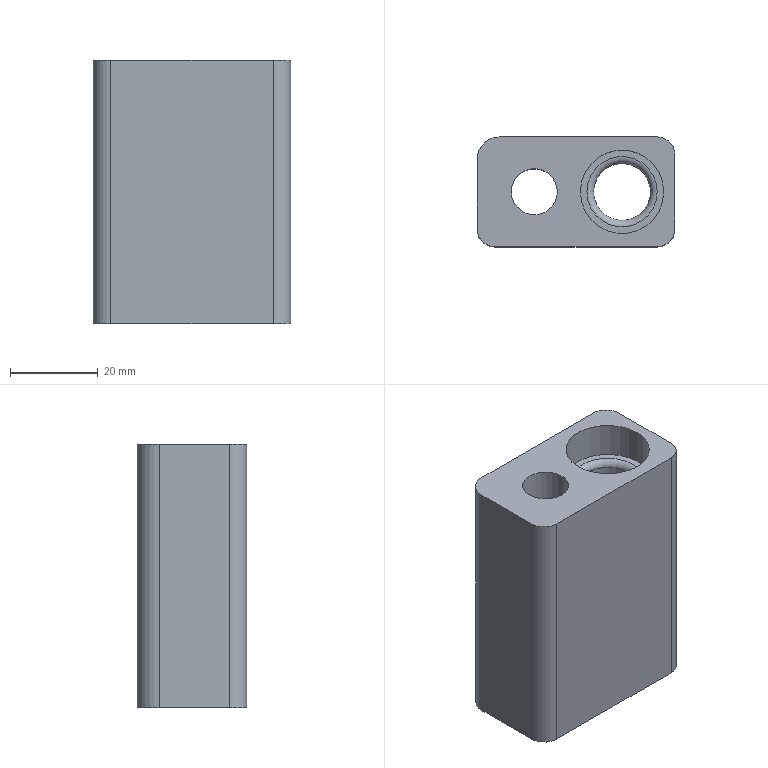Part | STEP file | gslz 2016.10.28-10_id2346_x_t | 1 solid | 17 faces | box 45 x 25 x 60 mm | volume 46550 mm3 | plane 8 | cylinder 8 | torus 1 | commonest cylinder face diameters 8 x3 10 x1 10.5 x1 13 x1 17 x1 19 x1
STEP:
#1=CARTESIAN_POINT('',(0.,0.,0.));
#2=DIRECTION('',(0.,0.,1.));
#3=DIRECTION('',(1.,0.,0.));
#4=AXIS2_PLACEMENT_3D('',#1,#2,#3);
#5=CARTESIAN_POINT('',(1091.668,100.693,85.));
#6=VERTEX_POINT('',#5);
#7=CARTESIAN_POINT('',(1082.168,100.693,85.));
#8=DIRECTION('',(0.,0.,1.));
#9=DIRECTION('',(1.,0.,0.));
#10=AXIS2_PLACEMENT_3D('',#7,#8,#9);
#11=CIRCLE('',#10,9.5);
#12=CARTESIAN_POINT('',(1123.168,94.693,85.));
#13=DIRECTION('',(0.,0.,1.));
#14=DIRECTION('',(-1.,0.,0.));
#15=AXIS2_PLACEMENT_3D('',#12,#13,#14);
#16=PLANE('',#15);
#17=CARTESIAN_POINT('',(41.,-6.));
#18=DIRECTION('',(-1.,0.));
#19=AXIS2_PLACEMENT_2D('',#17,#18);
#20=CIRCLE('',#19,9.5);
#21=(GEOMETRIC_REPRESENTATION_CONTEXT(2)PARAMETRIC_REPRESENTATION_CONTEXT()REPRESENTATION_CONTEXT('',''));
#22=DEFINITIONAL_REPRESENTATION('',(#20),#21);
#23=PCURVE('',#16,#22);
#24=CARTESIAN_POINT('',(1082.168,100.693,81.));
#25=DIRECTION('',(0.,0.,-1.));
#26=DIRECTION('',(-1.,0.,0.));
#27=AXIS2_PLACEMENT_3D('',#24,#25,#26);
#28=CYLINDRICAL_SURFACE('',#27,9.5);
#29=CARTESIAN_POINT('',(9.425,-4.));
#30=DIRECTION('',(-1.,0.));
#31=VECTOR('',#30,1.);
#32=LINE('',#29,#31);
#33=(GEOMETRIC_REPRESENTATION_CONTEXT(2)PARAMETRIC_REPRESENTATION_CONTEXT()REPRESENTATION_CONTEXT('',''));
#34=DEFINITIONAL_REPRESENTATION('',(#32),#33);
#35=PCURVE('',#28,#34);
#36=SURFACE_CURVE('',#11,(#23,#35),.PCURVE_S1.);
#37=EDGE_CURVE('',#6,#6,#36,.T.);
#38=ORIENTED_EDGE('',*,*,#37,.F.);
#39=EDGE_LOOP('',(#38));
#40=FACE_BOUND('',#39,.T.);
#41=CARTESIAN_POINT('',(1049.168,108.193,85.));
#42=VERTEX_POINT('',#41);
#43=CARTESIAN_POINT('',(1049.168,92.193,85.));
#44=VERTEX_POINT('',#43);
#45=CARTESIAN_POINT('',(1049.168,94.693,85.));
#46=DIRECTION('',(0.,-1.,0.));
#47=VECTOR('',#46,1.);
#48=LINE('',#45,#47);
#49=CARTESIAN_POINT('',(74.,0.));
#50=DIRECTION('',(0.,1.));
#51=VECTOR('',#50,1.);
#52=LINE('',#49,#51);
#53=(GEOMETRIC_REPRESENTATION_CONTEXT(2)PARAMETRIC_REPRESENTATION_CONTEXT()REPRESENTATION_CONTEXT('',''));
#54=DEFINITIONAL_REPRESENTATION('',(#52),#53);
#55=PCURVE('',#16,#54);
#56=CARTESIAN_POINT('',(1049.168,100.693,43.5));
#57=DIRECTION('',(-1.,0.,0.));
#58=DIRECTION('',(0.,0.,-1.));
#59=AXIS2_PLACEMENT_3D('',#56,#57,#58);
#60=PLANE('',#59);
#61=CARTESIAN_POINT('',(-41.5,6.));
#62=DIRECTION('',(0.,1.));
#63=VECTOR('',#62,1.);
#64=LINE('',#61,#63);
#65=(GEOMETRIC_REPRESENTATION_CONTEXT(2)PARAMETRIC_REPRESENTATION_CONTEXT()REPRESENTATION_CONTEXT('',''));
#66=DEFINITIONAL_REPRESENTATION('',(#64),#65);
#67=PCURVE('',#60,#66);
#68=SURFACE_CURVE('',#48,(#55,#67),.PCURVE_S1.);
#69=EDGE_CURVE('',#42,#44,#68,.T.);
#70=ORIENTED_EDGE('',*,*,#69,.T.);
#71=CARTESIAN_POINT('',(1053.168,88.193,85.));
#72=VERTEX_POINT('',#71);
#73=CARTESIAN_POINT('',(1053.168,92.193,85.));
#74=DIRECTION('',(0.,0.,1.));
#75=DIRECTION('',(1.,0.,0.));
#76=AXIS2_PLACEMENT_3D('',#73,#74,#75);
#77=CIRCLE('',#76,4.);
#78=CARTESIAN_POINT('',(70.,2.5));
#79=DIRECTION('',(-1.,0.));
#80=AXIS2_PLACEMENT_2D('',#78,#79);
#81=CIRCLE('',#80,4.);
#82=(GEOMETRIC_REPRESENTATION_CONTEXT(2)PARAMETRIC_REPRESENTATION_CONTEXT()REPRESENTATION_CONTEXT('',''));
#83=DEFINITIONAL_REPRESENTATION('',(#81),#82);
#84=PCURVE('',#16,#83);
#85=CARTESIAN_POINT('',(1053.168,92.193,43.5));
#86=DIRECTION('',(0.,0.,-1.));
#87=DIRECTION('',(1.,0.,0.));
#88=AXIS2_PLACEMENT_3D('',#85,#86,#87);
#89=CYLINDRICAL_SURFACE('',#88,4.);
#90=CARTESIAN_POINT('',(6.283,-41.5));
#91=DIRECTION('',(-1.,0.));
#92=VECTOR('',#91,1.);
#93=LINE('',#90,#92);
#94=(GEOMETRIC_REPRESENTATION_CONTEXT(2)PARAMETRIC_REPRESENTATION_CONTEXT()REPRESENTATION_CONTEXT('',''));
#95=DEFINITIONAL_REPRESENTATION('',(#93),#94);
#96=PCURVE('',#89,#95);
#97=SURFACE_CURVE('',#77,(#84,#96),.PCURVE_S1.);
#98=EDGE_CURVE('',#44,#72,#97,.T.);
#99=ORIENTED_EDGE('',*,*,#98,.T.);
#100=CARTESIAN_POINT('',(1090.168,88.193,85.));
#101=VERTEX_POINT('',#100);
#102=CARTESIAN_POINT('',(1165.804,88.193,85.));
#103=DIRECTION('',(1.,0.,0.));
#104=VECTOR('',#103,1.);
#105=LINE('',#102,#104);
#106=CARTESIAN_POINT('',(-42.635,6.5));
#107=DIRECTION('',(-1.,0.));
#108=VECTOR('',#107,1.);
#109=LINE('',#106,#108);
#110=(GEOMETRIC_REPRESENTATION_CONTEXT(2)PARAMETRIC_REPRESENTATION_CONTEXT()REPRESENTATION_CONTEXT('',''));
#111=DEFINITIONAL_REPRESENTATION('',(#109),#110);
#112=PCURVE('',#16,#111);
#113=CARTESIAN_POINT('',(1165.804,88.193,80.));
#114=DIRECTION('',(0.,1.,0.));
#115=DIRECTION('',(0.,0.,-1.));
#116=AXIS2_PLACEMENT_3D('',#113,#114,#115);
#117=PLANE('',#116);
#118=CARTESIAN_POINT('',(-5.,0.));
#119=DIRECTION('',(0.,-1.));
#120=VECTOR('',#119,1.);
#121=LINE('',#118,#120);
#122=(GEOMETRIC_REPRESENTATION_CONTEXT(2)PARAMETRIC_REPRESENTATION_CONTEXT()REPRESENTATION_CONTEXT('',''));
#123=DEFINITIONAL_REPRESENTATION('',(#121),#122);
#124=PCURVE('',#117,#123);
#125=SURFACE_CURVE('',#105,(#112,#124),.PCURVE_S1.);
#126=EDGE_CURVE('',#72,#101,#125,.T.);
#127=ORIENTED_EDGE('',*,*,#126,.T.);
#128=CARTESIAN_POINT('',(1094.168,92.193,85.));
#129=VERTEX_POINT('',#128);
#130=CARTESIAN_POINT('',(1090.168,92.193,85.));
#131=DIRECTION('',(0.,0.,1.));
#132=DIRECTION('',(1.,0.,0.));
#133=AXIS2_PLACEMENT_3D('',#130,#131,#132);
#134=CIRCLE('',#133,4.);
#135=CARTESIAN_POINT('',(33.,2.5));
#136=DIRECTION('',(-1.,0.));
#137=AXIS2_PLACEMENT_2D('',#135,#136);
#138=CIRCLE('',#137,4.);
#139=(GEOMETRIC_REPRESENTATION_CONTEXT(2)PARAMETRIC_REPRESENTATION_CONTEXT()REPRESENTATION_CONTEXT('',''));
#140=DEFINITIONAL_REPRESENTATION('',(#138),#139);
#141=PCURVE('',#16,#140);
#142=CARTESIAN_POINT('',(1090.168,92.193,46.));
#143=DIRECTION('',(0.,0.,-1.));
#144=DIRECTION('',(1.,0.,0.));
#145=AXIS2_PLACEMENT_3D('',#142,#143,#144);
#146=CYLINDRICAL_SURFACE('',#145,4.);
#147=CARTESIAN_POINT('',(6.283,-39.));
#148=DIRECTION('',(-1.,0.));
#149=VECTOR('',#148,1.);
#150=LINE('',#147,#149);
#151=(GEOMETRIC_REPRESENTATION_CONTEXT(2)PARAMETRIC_REPRESENTATION_CONTEXT()REPRESENTATION_CONTEXT('',''));
#152=DEFINITIONAL_REPRESENTATION('',(#150),#151);
#153=PCURVE('',#146,#152);
#154=SURFACE_CURVE('',#134,(#141,#153),.PCURVE_S1.);
#155=EDGE_CURVE('',#101,#129,#154,.T.);
#156=ORIENTED_EDGE('',*,*,#155,.T.);
#157=CARTESIAN_POINT('',(1094.168,109.193,85.));
#158=VERTEX_POINT('',#157);
#159=CARTESIAN_POINT('',(1094.168,100.693,85.));
#160=DIRECTION('',(0.,1.,0.));
#161=VECTOR('',#160,1.);
#162=LINE('',#159,#161);
#163=CARTESIAN_POINT('',(29.,-6.));
#164=DIRECTION('',(0.,-1.));
#165=VECTOR('',#164,1.);
#166=LINE('',#163,#165);
#167=(GEOMETRIC_REPRESENTATION_CONTEXT(2)PARAMETRIC_REPRESENTATION_CONTEXT()REPRESENTATION_CONTEXT('',''));
#168=DEFINITIONAL_REPRESENTATION('',(#166),#167);
#169=PCURVE('',#16,#168);
#170=CARTESIAN_POINT('',(1094.168,100.693,46.));
#171=DIRECTION('',(-1.,0.,0.));
#172=DIRECTION('',(0.,0.,-1.));
#173=AXIS2_PLACEMENT_3D('',#170,#171,#172);
#174=PLANE('',#173);
#175=CARTESIAN_POINT('',(-39.,0.));
#176=DIRECTION('',(0.,-1.));
#177=VECTOR('',#176,1.);
#178=LINE('',#175,#177);
#179=(GEOMETRIC_REPRESENTATION_CONTEXT(2)PARAMETRIC_REPRESENTATION_CONTEXT()REPRESENTATION_CONTEXT('',''));
#180=DEFINITIONAL_REPRESENTATION('',(#178),#179);
#181=PCURVE('',#174,#180);
#182=SURFACE_CURVE('',#162,(#169,#181),.PCURVE_S1.);
#183=EDGE_CURVE('',#129,#158,#182,.T.);
#184=ORIENTED_EDGE('',*,*,#183,.T.);
#185=CARTESIAN_POINT('',(1090.168,113.193,85.));
#186=VERTEX_POINT('',#185);
#187=CARTESIAN_POINT('',(1090.168,109.193,85.));
#188=DIRECTION('',(0.,0.,1.));
#189=DIRECTION('',(1.,0.,0.));
#190=AXIS2_PLACEMENT_3D('',#187,#188,#189);
#191=CIRCLE('',#190,4.);
#192=CARTESIAN_POINT('',(33.,-14.5));
#193=DIRECTION('',(-1.,0.));
#194=AXIS2_PLACEMENT_2D('',#192,#193);
#195=CIRCLE('',#194,4.);
#196=(GEOMETRIC_REPRESENTATION_CONTEXT(2)PARAMETRIC_REPRESENTATION_CONTEXT()REPRESENTATION_CONTEXT('',''));
#197=DEFINITIONAL_REPRESENTATION('',(#195),#196);
#198=PCURVE('',#16,#197);
#199=CARTESIAN_POINT('',(1090.168,109.193,80.));
#200=DIRECTION('',(0.,0.,-1.));
#201=DIRECTION('',(1.,0.,0.));
#202=AXIS2_PLACEMENT_3D('',#199,#200,#201);
#203=CYLINDRICAL_SURFACE('',#202,4.);
#204=CARTESIAN_POINT('',(6.283,-5.));
#205=DIRECTION('',(-1.,0.));
#206=VECTOR('',#205,1.);
#207=LINE('',#204,#206);
#208=(GEOMETRIC_REPRESENTATION_CONTEXT(2)PARAMETRIC_REPRESENTATION_CONTEXT()REPRESENTATION_CONTEXT('',''));
#209=DEFINITIONAL_REPRESENTATION('',(#207),#208);
#210=PCURVE('',#203,#209);
#211=SURFACE_CURVE('',#191,(#198,#210),.PCURVE_S1.);
#212=EDGE_CURVE('',#158,#186,#211,.T.);
#213=ORIENTED_EDGE('',*,*,#212,.T.);
#214=CARTESIAN_POINT('',(1054.168,113.193,85.));
#215=VERTEX_POINT('',#214);
#216=CARTESIAN_POINT('',(430.168,113.193,85.));
#217=DIRECTION('',(-1.,0.,0.));
#218=VECTOR('',#217,1.);
#219=LINE('',#216,#218);
#220=CARTESIAN_POINT('',(693.,-18.5));
#221=DIRECTION('',(1.,0.));
#222=VECTOR('',#221,1.);
#223=LINE('',#220,#222);
#224=(GEOMETRIC_REPRESENTATION_CONTEXT(2)PARAMETRIC_REPRESENTATION_CONTEXT()REPRESENTATION_CONTEXT('',''));
#225=DEFINITIONAL_REPRESENTATION('',(#223),#224);
#226=PCURVE('',#16,#225);
#227=CARTESIAN_POINT('',(430.168,113.193,80.));
#228=DIRECTION('',(0.,-1.,0.));
#229=DIRECTION('',(0.,0.,1.));
#230=AXIS2_PLACEMENT_3D('',#227,#228,#229);
#231=PLANE('',#230);
#232=CARTESIAN_POINT('',(5.,0.));
#233=DIRECTION('',(0.,1.));
#234=VECTOR('',#233,1.);
#235=LINE('',#232,#234);
#236=(GEOMETRIC_REPRESENTATION_CONTEXT(2)PARAMETRIC_REPRESENTATION_CONTEXT()REPRESENTATION_CONTEXT('',''));
#237=DEFINITIONAL_REPRESENTATION('',(#235),#236);
#238=PCURVE('',#231,#237);
#239=SURFACE_CURVE('',#219,(#226,#238),.PCURVE_S1.);
#240=EDGE_CURVE('',#186,#215,#239,.T.);
#241=ORIENTED_EDGE('',*,*,#240,.T.);
#242=CARTESIAN_POINT('',(1054.168,108.193,85.));
#243=DIRECTION('',(0.,0.,1.));
#244=DIRECTION('',(1.,0.,0.));
#245=AXIS2_PLACEMENT_3D('',#242,#243,#244);
#246=CIRCLE('',#245,5.);
#247=CARTESIAN_POINT('',(69.,-13.5));
#248=DIRECTION('',(-1.,0.));
#249=AXIS2_PLACEMENT_2D('',#247,#248);
#250=CIRCLE('',#249,5.);
#251=(GEOMETRIC_REPRESENTATION_CONTEXT(2)PARAMETRIC_REPRESENTATION_CONTEXT()REPRESENTATION_CONTEXT('',''));
#252=DEFINITIONAL_REPRESENTATION('',(#250),#251);
#253=PCURVE('',#16,#252);
#254=CARTESIAN_POINT('',(1054.168,108.193,43.5));
#255=DIRECTION('',(0.,0.,1.));
#256=DIRECTION('',(-1.,0.,0.));
#257=AXIS2_PLACEMENT_3D('',#254,#255,#256);
#258=CYLINDRICAL_SURFACE('',#257,5.);
#259=CARTESIAN_POINT('',(3.142,41.5));
#260=DIRECTION('',(1.,0.));
#261=VECTOR('',#260,1.);
#262=LINE('',#259,#261);
#263=(GEOMETRIC_REPRESENTATION_CONTEXT(2)PARAMETRIC_REPRESENTATION_CONTEXT()REPRESENTATION_CONTEXT('',''));
#264=DEFINITIONAL_REPRESENTATION('',(#262),#263);
#265=PCURVE('',#258,#264);
#266=SURFACE_CURVE('',#246,(#253,#265),.PCURVE_S1.);
#267=EDGE_CURVE('',#215,#42,#266,.T.);
#268=ORIENTED_EDGE('',*,*,#267,.T.);
#269=EDGE_LOOP('',(#70,#99,#127,#156,#184,#213,#241,#268));
#270=FACE_BOUND('',#269,.T.);
#271=CARTESIAN_POINT('',(1067.418,100.693,85.));
#272=VERTEX_POINT('',#271);
#273=CARTESIAN_POINT('',(1062.168,100.693,85.));
#274=DIRECTION('',(0.,0.,-1.));
#275=DIRECTION('',(1.,0.,0.));
#276=AXIS2_PLACEMENT_3D('',#273,#274,#275);
#277=CIRCLE('',#276,5.25);
#278=CARTESIAN_POINT('',(55.75,-6.));
#279=CARTESIAN_POINT('',(55.75,3.093));
#280=CARTESIAN_POINT('',(63.625,-1.453));
#281=CARTESIAN_POINT('',(71.5,-6.));
#282=CARTESIAN_POINT('',(63.625,-10.547));
#283=CARTESIAN_POINT('',(55.75,-15.093));
#284=CARTESIAN_POINT('',(55.75,-6.));
#285=(BOUNDED_CURVE()B_SPLINE_CURVE(2,(#278,#279,#280,#281,#282,#283,#284),.UNSPECIFIED.,.T.,.F.)B_SPLINE_CURVE_WITH_KNOTS((1,2,2,2,2,1),(-2.094,0.,2.094,4.189,6.283,8.378),.UNSPECIFIED.)CURVE()GEOMETRIC_REPRESENTATION_ITEM()RATIONAL_B_SPLINE_CURVE((1.,0.5,1.,0.5,1.,0.5,1.))REPRESENTATION_ITEM(''));
#286=(GEOMETRIC_REPRESENTATION_CONTEXT(2)PARAMETRIC_REPRESENTATION_CONTEXT()REPRESENTATION_CONTEXT('',''));
#287=DEFINITIONAL_REPRESENTATION('',(#285),#286);
#288=PCURVE('',#16,#287);
#289=CARTESIAN_POINT('',(1062.168,100.693,-18.));
#290=DIRECTION('',(0.,0.,1.));
#291=DIRECTION('',(-1.,0.,0.));
#292=AXIS2_PLACEMENT_3D('',#289,#290,#291);
#293=CYLINDRICAL_SURFACE('',#292,5.25);
#294=CARTESIAN_POINT('',(9.425,103.));
#295=DIRECTION('',(-1.,0.));
#296=VECTOR('',#295,1.);
#297=LINE('',#294,#296);
#298=(GEOMETRIC_REPRESENTATION_CONTEXT(2)PARAMETRIC_REPRESENTATION_CONTEXT()REPRESENTATION_CONTEXT('',''));
#299=DEFINITIONAL_REPRESENTATION('',(#297),#298);
#300=PCURVE('',#293,#299);
#301=SURFACE_CURVE('',#277,(#288,#300),.PCURVE_S1.);
#302=EDGE_CURVE('',#272,#272,#301,.T.);
#303=ORIENTED_EDGE('',*,*,#302,.T.);
#304=EDGE_LOOP('',(#303));
#305=FACE_BOUND('',#304,.T.);
#306=ADVANCED_FACE('',(#40,#270,#305),#16,.T.);
#307=CARTESIAN_POINT('',(1075.668,100.693,25.));
#308=VERTEX_POINT('',#307);
#309=CARTESIAN_POINT('',(1082.168,100.693,25.));
#310=DIRECTION('',(0.,0.,1.));
#311=DIRECTION('',(-1.,0.,0.));
#312=AXIS2_PLACEMENT_3D('',#309,#310,#311);
#313=CIRCLE('',#312,6.5);
#314=CARTESIAN_POINT('',(1131.168,154.693,25.));
#315=DIRECTION('',(0.,0.,-1.));
#316=DIRECTION('',(1.,0.,0.));
#317=AXIS2_PLACEMENT_3D('',#314,#315,#316);
#318=PLANE('',#317);
#319=CARTESIAN_POINT('',(-55.5,54.));
#320=CARTESIAN_POINT('',(-55.5,65.258));
#321=CARTESIAN_POINT('',(-45.75,59.629));
#322=CARTESIAN_POINT('',(-36.,54.));
#323=CARTESIAN_POINT('',(-45.75,48.371));
#324=CARTESIAN_POINT('',(-55.5,42.742));
#325=CARTESIAN_POINT('',(-55.5,54.));
#326=(BOUNDED_CURVE()B_SPLINE_CURVE(2,(#319,#320,#321,#322,#323,#324,#325),.UNSPECIFIED.,.T.,.F.)B_SPLINE_CURVE_WITH_KNOTS((1,2,2,2,2,1),(-2.094,0.,2.094,4.189,6.283,8.378),.UNSPECIFIED.)CURVE()GEOMETRIC_REPRESENTATION_ITEM()RATIONAL_B_SPLINE_CURVE((1.,0.5,1.,0.5,1.,0.5,1.))REPRESENTATION_ITEM(''));
#327=(GEOMETRIC_REPRESENTATION_CONTEXT(2)PARAMETRIC_REPRESENTATION_CONTEXT()REPRESENTATION_CONTEXT('',''));
#328=DEFINITIONAL_REPRESENTATION('',(#326),#327);
#329=PCURVE('',#318,#328);
#330=CARTESIAN_POINT('',(1082.168,100.693,45.5));
#331=DIRECTION('',(0.,0.,-1.));
#332=DIRECTION('',(-1.,0.,0.));
#333=AXIS2_PLACEMENT_3D('',#330,#331,#332);
#334=CYLINDRICAL_SURFACE('',#333,6.5);
#335=CARTESIAN_POINT('',(6.283,20.5));
#336=DIRECTION('',(-1.,0.));
#337=VECTOR('',#336,1.);
#338=LINE('',#335,#337);
#339=(GEOMETRIC_REPRESENTATION_CONTEXT(2)PARAMETRIC_REPRESENTATION_CONTEXT()REPRESENTATION_CONTEXT('',''));
#340=DEFINITIONAL_REPRESENTATION('',(#338),#339);
#341=PCURVE('',#334,#340);
#342=SURFACE_CURVE('',#313,(#329,#341),.PCURVE_S1.);
#343=EDGE_CURVE('',#308,#308,#342,.T.);
#344=ORIENTED_EDGE('',*,*,#343,.T.);
#345=EDGE_LOOP('',(#344));
#346=FACE_BOUND('',#345,.T.);
#347=CARTESIAN_POINT('',(1053.668,100.693,25.));
#348=VERTEX_POINT('',#347);
#349=CARTESIAN_POINT('',(1062.168,100.693,25.));
#350=DIRECTION('',(0.,0.,1.));
#351=DIRECTION('',(-1.,0.,0.));
#352=AXIS2_PLACEMENT_3D('',#349,#350,#351);
#353=CIRCLE('',#352,8.5);
#354=CARTESIAN_POINT('',(-77.5,54.));
#355=CARTESIAN_POINT('',(-77.5,68.722));
#356=CARTESIAN_POINT('',(-64.75,61.361));
#357=CARTESIAN_POINT('',(-52.,54.));
#358=CARTESIAN_POINT('',(-64.75,46.639));
#359=CARTESIAN_POINT('',(-77.5,39.278));
#360=CARTESIAN_POINT('',(-77.5,54.));
#361=(BOUNDED_CURVE()B_SPLINE_CURVE(2,(#354,#355,#356,#357,#358,#359,#360),.UNSPECIFIED.,.T.,.F.)B_SPLINE_CURVE_WITH_KNOTS((1,2,2,2,2,1),(-2.094,0.,2.094,4.189,6.283,8.378),.UNSPECIFIED.)CURVE()GEOMETRIC_REPRESENTATION_ITEM()RATIONAL_B_SPLINE_CURVE((1.,0.5,1.,0.5,1.,0.5,1.))REPRESENTATION_ITEM(''));
#362=(GEOMETRIC_REPRESENTATION_CONTEXT(2)PARAMETRIC_REPRESENTATION_CONTEXT()REPRESENTATION_CONTEXT('',''));
#363=DEFINITIONAL_REPRESENTATION('',(#361),#362);
#364=PCURVE('',#318,#363);
#365=CARTESIAN_POINT('',(1062.168,100.693,-8.));
#366=DIRECTION('',(0.,0.,1.));
#367=DIRECTION('',(-1.,0.,0.));
#368=AXIS2_PLACEMENT_3D('',#365,#366,#367);
#369=CYLINDRICAL_SURFACE('',#368,8.5);
#370=CARTESIAN_POINT('',(0.,33.));
#371=DIRECTION('',(1.,0.));
#372=VECTOR('',#371,1.);
#373=LINE('',#370,#372);
#374=(GEOMETRIC_REPRESENTATION_CONTEXT(2)PARAMETRIC_REPRESENTATION_CONTEXT()REPRESENTATION_CONTEXT('',''));
#375=DEFINITIONAL_REPRESENTATION('',(#373),#374);
#376=PCURVE('',#369,#375);
#377=SURFACE_CURVE('',#353,(#364,#376),.PCURVE_S1.);
#378=EDGE_CURVE('',#348,#348,#377,.T.);
#379=ORIENTED_EDGE('',*,*,#378,.T.);
#380=EDGE_LOOP('',(#379));
#381=FACE_BOUND('',#380,.T.);
#382=CARTESIAN_POINT('',(1053.168,88.193,25.));
#383=VERTEX_POINT('',#382);
#384=CARTESIAN_POINT('',(1090.168,88.193,25.));
#385=VERTEX_POINT('',#384);
#386=CARTESIAN_POINT('',(1131.168,88.193,25.));
#387=DIRECTION('',(1.,0.,0.));
#388=VECTOR('',#387,1.);
#389=LINE('',#386,#388);
#390=CARTESIAN_POINT('',(0.,66.5));
#391=DIRECTION('',(1.,0.));
#392=VECTOR('',#391,1.);
#393=LINE('',#390,#392);
#394=(GEOMETRIC_REPRESENTATION_CONTEXT(2)PARAMETRIC_REPRESENTATION_CONTEXT()REPRESENTATION_CONTEXT('',''));
#395=DEFINITIONAL_REPRESENTATION('',(#393),#394);
#396=PCURVE('',#318,#395);
#397=CARTESIAN_POINT('',(55.,34.635));
#398=DIRECTION('',(0.,-1.));
#399=VECTOR('',#398,1.);
#400=LINE('',#397,#399);
#401=(GEOMETRIC_REPRESENTATION_CONTEXT(2)PARAMETRIC_REPRESENTATION_CONTEXT()REPRESENTATION_CONTEXT('',''));
#402=DEFINITIONAL_REPRESENTATION('',(#400),#401);
#403=PCURVE('',#117,#402);
#404=SURFACE_CURVE('',#389,(#396,#403),.PCURVE_S1.);
#405=EDGE_CURVE('',#383,#385,#404,.T.);
#406=ORIENTED_EDGE('',*,*,#405,.F.);
#407=CARTESIAN_POINT('',(1049.168,92.193,25.));
#408=VERTEX_POINT('',#407);
#409=CARTESIAN_POINT('',(1053.168,92.193,25.));
#410=DIRECTION('',(0.,0.,-1.));
#411=DIRECTION('',(-1.,0.,0.));
#412=AXIS2_PLACEMENT_3D('',#409,#410,#411);
#413=CIRCLE('',#412,4.);
#414=CARTESIAN_POINT('',(-78.,62.5));
#415=DIRECTION('',(-1.,0.));
#416=AXIS2_PLACEMENT_2D('',#414,#415);
#417=CIRCLE('',#416,4.);
#418=(GEOMETRIC_REPRESENTATION_CONTEXT(2)PARAMETRIC_REPRESENTATION_CONTEXT()REPRESENTATION_CONTEXT('',''));
#419=DEFINITIONAL_REPRESENTATION('',(#417),#418);
#420=PCURVE('',#318,#419);
#421=CARTESIAN_POINT('',(-3.142,18.5));
#422=DIRECTION('',(1.,0.));
#423=VECTOR('',#422,1.);
#424=LINE('',#421,#423);
#425=(GEOMETRIC_REPRESENTATION_CONTEXT(2)PARAMETRIC_REPRESENTATION_CONTEXT()REPRESENTATION_CONTEXT('',''));
#426=DEFINITIONAL_REPRESENTATION('',(#424),#425);
#427=PCURVE('',#89,#426);
#428=SURFACE_CURVE('',#413,(#420,#427),.PCURVE_S1.);
#429=EDGE_CURVE('',#383,#408,#428,.T.);
#430=ORIENTED_EDGE('',*,*,#429,.T.);
#431=CARTESIAN_POINT('',(1049.168,108.193,25.));
#432=VERTEX_POINT('',#431);
#433=CARTESIAN_POINT('',(1049.168,154.693,25.));
#434=DIRECTION('',(0.,1.,0.));
#435=VECTOR('',#434,1.);
#436=LINE('',#433,#435);
#437=CARTESIAN_POINT('',(-82.,0.));
#438=DIRECTION('',(0.,-1.));
#439=VECTOR('',#438,1.);
#440=LINE('',#437,#439);
#441=(GEOMETRIC_REPRESENTATION_CONTEXT(2)PARAMETRIC_REPRESENTATION_CONTEXT()REPRESENTATION_CONTEXT('',''));
#442=DEFINITIONAL_REPRESENTATION('',(#440),#441);
#443=PCURVE('',#318,#442);
#444=CARTESIAN_POINT('',(18.5,-54.));
#445=DIRECTION('',(0.,-1.));
#446=VECTOR('',#445,1.);
#447=LINE('',#444,#446);
#448=(GEOMETRIC_REPRESENTATION_CONTEXT(2)PARAMETRIC_REPRESENTATION_CONTEXT()REPRESENTATION_CONTEXT('',''));
#449=DEFINITIONAL_REPRESENTATION('',(#447),#448);
#450=PCURVE('',#60,#449);
#451=SURFACE_CURVE('',#436,(#443,#450),.PCURVE_S1.);
#452=EDGE_CURVE('',#408,#432,#451,.T.);
#453=ORIENTED_EDGE('',*,*,#452,.T.);
#454=CARTESIAN_POINT('',(1054.168,113.193,25.));
#455=VERTEX_POINT('',#454);
#456=CARTESIAN_POINT('',(1054.168,108.193,25.));
#457=DIRECTION('',(0.,0.,-1.));
#458=DIRECTION('',(-1.,0.,0.));
#459=AXIS2_PLACEMENT_3D('',#456,#457,#458);
#460=CIRCLE('',#459,5.);
#461=CARTESIAN_POINT('',(-77.,46.5));
#462=DIRECTION('',(-1.,0.));
#463=AXIS2_PLACEMENT_2D('',#461,#462);
#464=CIRCLE('',#463,5.);
#465=(GEOMETRIC_REPRESENTATION_CONTEXT(2)PARAMETRIC_REPRESENTATION_CONTEXT()REPRESENTATION_CONTEXT('',''));
#466=DEFINITIONAL_REPRESENTATION('',(#464),#465);
#467=PCURVE('',#318,#466);
#468=CARTESIAN_POINT('',(6.283,-18.5));
#469=DIRECTION('',(-1.,0.));
#470=VECTOR('',#469,1.);
#471=LINE('',#468,#470);
#472=(GEOMETRIC_REPRESENTATION_CONTEXT(2)PARAMETRIC_REPRESENTATION_CONTEXT()REPRESENTATION_CONTEXT('',''));
#473=DEFINITIONAL_REPRESENTATION('',(#471),#472);
#474=PCURVE('',#258,#473);
#475=SURFACE_CURVE('',#460,(#467,#474),.PCURVE_S1.);
#476=EDGE_CURVE('',#432,#455,#475,.T.);
#477=ORIENTED_EDGE('',*,*,#476,.T.);
#478=CARTESIAN_POINT('',(1090.168,113.193,25.));
#479=VERTEX_POINT('',#478);
#480=CARTESIAN_POINT('',(1131.168,113.193,25.));
#481=DIRECTION('',(-1.,0.,0.));
#482=VECTOR('',#481,1.);
#483=LINE('',#480,#482);
#484=CARTESIAN_POINT('',(0.,41.5));
#485=DIRECTION('',(-1.,0.));
#486=VECTOR('',#485,1.);
#487=LINE('',#484,#486);
#488=(GEOMETRIC_REPRESENTATION_CONTEXT(2)PARAMETRIC_REPRESENTATION_CONTEXT()REPRESENTATION_CONTEXT('',''));
#489=DEFINITIONAL_REPRESENTATION('',(#487),#488);
#490=PCURVE('',#318,#489);
#491=CARTESIAN_POINT('',(-55.,-701.));
#492=DIRECTION('',(0.,1.));
#493=VECTOR('',#492,1.);
#494=LINE('',#491,#493);
#495=(GEOMETRIC_REPRESENTATION_CONTEXT(2)PARAMETRIC_REPRESENTATION_CONTEXT()REPRESENTATION_CONTEXT('',''));
#496=DEFINITIONAL_REPRESENTATION('',(#494),#495);
#497=PCURVE('',#231,#496);
#498=SURFACE_CURVE('',#483,(#490,#497),.PCURVE_S1.);
#499=EDGE_CURVE('',#479,#455,#498,.T.);
#500=ORIENTED_EDGE('',*,*,#499,.F.);
#501=CARTESIAN_POINT('',(1094.168,109.193,25.));
#502=VERTEX_POINT('',#501);
#503=CARTESIAN_POINT('',(1090.168,109.193,25.));
#504=DIRECTION('',(0.,0.,-1.));
#505=DIRECTION('',(-1.,0.,0.));
#506=AXIS2_PLACEMENT_3D('',#503,#504,#505);
#507=CIRCLE('',#506,4.);
#508=CARTESIAN_POINT('',(-41.,45.5));
#509=DIRECTION('',(-1.,0.));
#510=AXIS2_PLACEMENT_2D('',#508,#509);
#511=CIRCLE('',#510,4.);
#512=(GEOMETRIC_REPRESENTATION_CONTEXT(2)PARAMETRIC_REPRESENTATION_CONTEXT()REPRESENTATION_CONTEXT('',''));
#513=DEFINITIONAL_REPRESENTATION('',(#511),#512);
#514=PCURVE('',#318,#513);
#515=CARTESIAN_POINT('',(3.142,55.));
#516=DIRECTION('',(1.,0.));
#517=VECTOR('',#516,1.);
#518=LINE('',#515,#517);
#519=(GEOMETRIC_REPRESENTATION_CONTEXT(2)PARAMETRIC_REPRESENTATION_CONTEXT()REPRESENTATION_CONTEXT('',''));
#520=DEFINITIONAL_REPRESENTATION('',(#518),#519);
#521=PCURVE('',#203,#520);
#522=SURFACE_CURVE('',#507,(#514,#521),.PCURVE_S1.);
#523=EDGE_CURVE('',#479,#502,#522,.T.);
#524=ORIENTED_EDGE('',*,*,#523,.T.);
#525=CARTESIAN_POINT('',(1094.168,92.193,25.));
#526=VERTEX_POINT('',#525);
#527=CARTESIAN_POINT('',(1094.168,100.693,25.));
#528=DIRECTION('',(0.,-1.,0.));
#529=VECTOR('',#528,1.);
#530=LINE('',#527,#529);
#531=CARTESIAN_POINT('',(-37.,54.));
#532=DIRECTION('',(0.,1.));
#533=VECTOR('',#532,1.);
#534=LINE('',#531,#533);
#535=(GEOMETRIC_REPRESENTATION_CONTEXT(2)PARAMETRIC_REPRESENTATION_CONTEXT()REPRESENTATION_CONTEXT('',''));
#536=DEFINITIONAL_REPRESENTATION('',(#534),#535);
#537=PCURVE('',#318,#536);
#538=CARTESIAN_POINT('',(21.,0.));
#539=DIRECTION('',(0.,1.));
#540=VECTOR('',#539,1.);
#541=LINE('',#538,#540);
#542=(GEOMETRIC_REPRESENTATION_CONTEXT(2)PARAMETRIC_REPRESENTATION_CONTEXT()REPRESENTATION_CONTEXT('',''));
#543=DEFINITIONAL_REPRESENTATION('',(#541),#542);
#544=PCURVE('',#174,#543);
#545=SURFACE_CURVE('',#530,(#537,#544),.PCURVE_S1.);
#546=EDGE_CURVE('',#502,#526,#545,.T.);
#547=ORIENTED_EDGE('',*,*,#546,.T.);
#548=CARTESIAN_POINT('',(1090.168,92.193,25.));
#549=DIRECTION('',(0.,0.,-1.));
#550=DIRECTION('',(-1.,0.,0.));
#551=AXIS2_PLACEMENT_3D('',#548,#549,#550);
#552=CIRCLE('',#551,4.);
#553=CARTESIAN_POINT('',(-41.,62.5));
#554=DIRECTION('',(-1.,0.));
#555=AXIS2_PLACEMENT_2D('',#553,#554);
#556=CIRCLE('',#555,4.);
#557=(GEOMETRIC_REPRESENTATION_CONTEXT(2)PARAMETRIC_REPRESENTATION_CONTEXT()REPRESENTATION_CONTEXT('',''));
#558=DEFINITIONAL_REPRESENTATION('',(#556),#557);
#559=PCURVE('',#318,#558);
#560=CARTESIAN_POINT('',(-3.142,21.));
#561=DIRECTION('',(1.,0.));
#562=VECTOR('',#561,1.);
#563=LINE('',#560,#562);
#564=(GEOMETRIC_REPRESENTATION_CONTEXT(2)PARAMETRIC_REPRESENTATION_CONTEXT()REPRESENTATION_CONTEXT('',''));
#565=DEFINITIONAL_REPRESENTATION('',(#563),#564);
#566=PCURVE('',#146,#565);
#567=SURFACE_CURVE('',#552,(#559,#566),.PCURVE_S1.);
#568=EDGE_CURVE('',#526,#385,#567,.T.);
#569=ORIENTED_EDGE('',*,*,#568,.T.);
#570=EDGE_LOOP('',(#406,#430,#453,#477,#500,#524,#547,#569));
#571=FACE_BOUND('',#570,.T.);
#572=ADVANCED_FACE('',(#346,#381,#571),#318,.T.);
#573=ORIENTED_EDGE('',*,*,#499,.T.);
#574=CARTESIAN_POINT('',(1054.168,113.193,95.));
#575=DIRECTION('',(0.,0.,1.));
#576=VECTOR('',#575,1.);
#577=LINE('',#574,#576);
#578=CARTESIAN_POINT('',(15.,-624.));
#579=DIRECTION('',(1.,0.));
#580=VECTOR('',#579,1.);
#581=LINE('',#578,#580);
#582=(GEOMETRIC_REPRESENTATION_CONTEXT(2)PARAMETRIC_REPRESENTATION_CONTEXT()REPRESENTATION_CONTEXT('',''));
#583=DEFINITIONAL_REPRESENTATION('',(#581),#582);
#584=PCURVE('',#231,#583);
#585=CARTESIAN_POINT('',(4.712,51.5));
#586=DIRECTION('',(0.,1.));
#587=VECTOR('',#586,1.);
#588=LINE('',#585,#587);
#589=(GEOMETRIC_REPRESENTATION_CONTEXT(2)PARAMETRIC_REPRESENTATION_CONTEXT()REPRESENTATION_CONTEXT('',''));
#590=DEFINITIONAL_REPRESENTATION('',(#588),#589);
#591=PCURVE('',#258,#590);
#592=SURFACE_CURVE('',#577,(#584,#591),.PCURVE_S1.);
#593=EDGE_CURVE('',#455,#215,#592,.T.);
#594=ORIENTED_EDGE('',*,*,#593,.T.);
#595=ORIENTED_EDGE('',*,*,#240,.F.);
#596=CARTESIAN_POINT('',(1090.168,113.193,80.));
#597=DIRECTION('',(0.,0.,-1.));
#598=VECTOR('',#597,1.);
#599=LINE('',#596,#598);
#600=CARTESIAN_POINT('',(0.,-660.));
#601=DIRECTION('',(-1.,0.));
#602=VECTOR('',#601,1.);
#603=LINE('',#600,#602);
#604=(GEOMETRIC_REPRESENTATION_CONTEXT(2)PARAMETRIC_REPRESENTATION_CONTEXT()REPRESENTATION_CONTEXT('',''));
#605=DEFINITIONAL_REPRESENTATION('',(#603),#604);
#606=PCURVE('',#231,#605);
#607=CARTESIAN_POINT('',(4.712,0.));
#608=DIRECTION('',(0.,1.));
#609=VECTOR('',#608,1.);
#610=LINE('',#607,#609);
#611=(GEOMETRIC_REPRESENTATION_CONTEXT(2)PARAMETRIC_REPRESENTATION_CONTEXT()REPRESENTATION_CONTEXT('',''));
#612=DEFINITIONAL_REPRESENTATION('',(#610),#611);
#613=PCURVE('',#203,#612);
#614=SURFACE_CURVE('',#599,(#606,#613),.PCURVE_S1.);
#615=EDGE_CURVE('',#186,#479,#614,.T.);
#616=ORIENTED_EDGE('',*,*,#615,.T.);
#617=EDGE_LOOP('',(#573,#594,#595,#616));
#618=FACE_BOUND('',#617,.T.);
#619=ADVANCED_FACE('',(#618),#231,.F.);
#620=ORIENTED_EDGE('',*,*,#126,.F.);
#621=CARTESIAN_POINT('',(1053.168,88.193,43.5));
#622=DIRECTION('',(0.,0.,-1.));
#623=VECTOR('',#622,1.);
#624=LINE('',#621,#623);
#625=CARTESIAN_POINT('',(36.5,112.635));
#626=DIRECTION('',(1.,0.));
#627=VECTOR('',#626,1.);
#628=LINE('',#625,#627);
#629=(GEOMETRIC_REPRESENTATION_CONTEXT(2)PARAMETRIC_REPRESENTATION_CONTEXT()REPRESENTATION_CONTEXT('',''));
#630=DEFINITIONAL_REPRESENTATION('',(#628),#629);
#631=PCURVE('',#117,#630);
#632=CARTESIAN_POINT('',(1.571,0.));
#633=DIRECTION('',(0.,1.));
#634=VECTOR('',#633,1.);
#635=LINE('',#632,#634);
#636=(GEOMETRIC_REPRESENTATION_CONTEXT(2)PARAMETRIC_REPRESENTATION_CONTEXT()REPRESENTATION_CONTEXT('',''));
#637=DEFINITIONAL_REPRESENTATION('',(#635),#636);
#638=PCURVE('',#89,#637);
#639=SURFACE_CURVE('',#624,(#631,#638),.PCURVE_S1.);
#640=EDGE_CURVE('',#72,#383,#639,.T.);
#641=ORIENTED_EDGE('',*,*,#640,.T.);
#642=ORIENTED_EDGE('',*,*,#405,.T.);
#643=CARTESIAN_POINT('',(1090.168,88.193,80.));
#644=DIRECTION('',(0.,0.,1.));
#645=VECTOR('',#644,1.);
#646=LINE('',#643,#645);
#647=CARTESIAN_POINT('',(0.,75.635));
#648=DIRECTION('',(-1.,0.));
#649=VECTOR('',#648,1.);
#650=LINE('',#647,#649);
#651=(GEOMETRIC_REPRESENTATION_CONTEXT(2)PARAMETRIC_REPRESENTATION_CONTEXT()REPRESENTATION_CONTEXT('',''));
#652=DEFINITIONAL_REPRESENTATION('',(#650),#651);
#653=PCURVE('',#117,#652);
#654=CARTESIAN_POINT('',(1.571,-34.));
#655=DIRECTION('',(0.,-1.));
#656=VECTOR('',#655,1.);
#657=LINE('',#654,#656);
#658=(GEOMETRIC_REPRESENTATION_CONTEXT(2)PARAMETRIC_REPRESENTATION_CONTEXT()REPRESENTATION_CONTEXT('',''));
#659=DEFINITIONAL_REPRESENTATION('',(#657),#658);
#660=PCURVE('',#146,#659);
#661=SURFACE_CURVE('',#646,(#653,#660),.PCURVE_S1.);
#662=EDGE_CURVE('',#385,#101,#661,.T.);
#663=ORIENTED_EDGE('',*,*,#662,.T.);
#664=EDGE_LOOP('',(#620,#641,#642,#663));
#665=FACE_BOUND('',#664,.T.);
#666=ADVANCED_FACE('',(#665),#117,.F.);
#667=ORIENTED_EDGE('',*,*,#183,.F.);
#668=CARTESIAN_POINT('',(1094.168,92.193,46.));
#669=DIRECTION('',(0.,0.,-1.));
#670=VECTOR('',#669,1.);
#671=LINE('',#668,#670);
#672=CARTESIAN_POINT('',(0.,8.5));
#673=DIRECTION('',(1.,0.));
#674=VECTOR('',#673,1.);
#675=LINE('',#672,#674);
#676=(GEOMETRIC_REPRESENTATION_CONTEXT(2)PARAMETRIC_REPRESENTATION_CONTEXT()REPRESENTATION_CONTEXT('',''));
#677=DEFINITIONAL_REPRESENTATION('',(#675),#676);
#678=PCURVE('',#174,#677);
#679=CARTESIAN_POINT('',(0.,0.));
#680=DIRECTION('',(0.,1.));
#681=VECTOR('',#680,1.);
#682=LINE('',#679,#681);
#683=(GEOMETRIC_REPRESENTATION_CONTEXT(2)PARAMETRIC_REPRESENTATION_CONTEXT()REPRESENTATION_CONTEXT('',''));
#684=DEFINITIONAL_REPRESENTATION('',(#682),#683);
#685=PCURVE('',#146,#684);
#686=SURFACE_CURVE('',#671,(#678,#685),.PCURVE_S1.);
#687=EDGE_CURVE('',#129,#526,#686,.T.);
#688=ORIENTED_EDGE('',*,*,#687,.T.);
#689=ORIENTED_EDGE('',*,*,#546,.F.);
#690=CARTESIAN_POINT('',(1094.168,109.193,46.));
#691=DIRECTION('',(0.,0.,1.));
#692=VECTOR('',#691,1.);
#693=LINE('',#690,#692);
#694=CARTESIAN_POINT('',(0.,-8.5));
#695=DIRECTION('',(-1.,0.));
#696=VECTOR('',#695,1.);
#697=LINE('',#694,#696);
#698=(GEOMETRIC_REPRESENTATION_CONTEXT(2)PARAMETRIC_REPRESENTATION_CONTEXT()REPRESENTATION_CONTEXT('',''));
#699=DEFINITIONAL_REPRESENTATION('',(#697),#698);
#700=PCURVE('',#174,#699);
#701=CARTESIAN_POINT('',(6.283,34.));
#702=DIRECTION('',(0.,-1.));
#703=VECTOR('',#702,1.);
#704=LINE('',#701,#703);
#705=(GEOMETRIC_REPRESENTATION_CONTEXT(2)PARAMETRIC_REPRESENTATION_CONTEXT()REPRESENTATION_CONTEXT('',''));
#706=DEFINITIONAL_REPRESENTATION('',(#704),#705);
#707=PCURVE('',#203,#706);
#708=SURFACE_CURVE('',#693,(#700,#707),.PCURVE_S1.);
#709=EDGE_CURVE('',#502,#158,#708,.T.);
#710=ORIENTED_EDGE('',*,*,#709,.T.);
#711=EDGE_LOOP('',(#667,#688,#689,#710));
#712=FACE_BOUND('',#711,.T.);
#713=ADVANCED_FACE('',(#712),#174,.F.);
#714=ORIENTED_EDGE('',*,*,#568,.F.);
#715=ORIENTED_EDGE('',*,*,#687,.F.);
#716=ORIENTED_EDGE('',*,*,#155,.F.);
#717=ORIENTED_EDGE('',*,*,#662,.F.);
#718=EDGE_LOOP('',(#714,#715,#716,#717));
#719=FACE_BOUND('',#718,.T.);
#720=ADVANCED_FACE('',(#719),#146,.T.);
#721=ORIENTED_EDGE('',*,*,#523,.F.);
#722=ORIENTED_EDGE('',*,*,#615,.F.);
#723=ORIENTED_EDGE('',*,*,#212,.F.);
#724=ORIENTED_EDGE('',*,*,#709,.F.);
#725=EDGE_LOOP('',(#721,#722,#723,#724));
#726=FACE_BOUND('',#725,.T.);
#727=ADVANCED_FACE('',(#726),#203,.T.);
#728=CARTESIAN_POINT('',(1067.418,100.693,65.));
#729=VERTEX_POINT('',#728);
#730=CARTESIAN_POINT('',(1062.168,100.693,65.));
#731=DIRECTION('',(0.,0.,1.));
#732=DIRECTION('',(1.,0.,0.));
#733=AXIS2_PLACEMENT_3D('',#730,#731,#732);
#734=CIRCLE('',#733,5.25);
#735=CARTESIAN_POINT('',(3.142,83.));
#736=DIRECTION('',(1.,0.));
#737=VECTOR('',#736,1.);
#738=LINE('',#735,#737);
#739=(GEOMETRIC_REPRESENTATION_CONTEXT(2)PARAMETRIC_REPRESENTATION_CONTEXT()REPRESENTATION_CONTEXT('',''));
#740=DEFINITIONAL_REPRESENTATION('',(#738),#739);
#741=PCURVE('',#293,#740);
#742=CARTESIAN_POINT('',(389.238,18.295,65.));
#743=DIRECTION('',(0.,0.,1.));
#744=DIRECTION('',(-1.,0.,0.));
#745=AXIS2_PLACEMENT_3D('',#742,#743,#744);
#746=PLANE('',#745);
#747=CARTESIAN_POINT('',(-672.93,-82.398));
#748=DIRECTION('',(-1.,0.));
#749=AXIS2_PLACEMENT_2D('',#747,#748);
#750=CIRCLE('',#749,5.25);
#751=(GEOMETRIC_REPRESENTATION_CONTEXT(2)PARAMETRIC_REPRESENTATION_CONTEXT()REPRESENTATION_CONTEXT('',''));
#752=DEFINITIONAL_REPRESENTATION('',(#750),#751);
#753=PCURVE('',#746,#752);
#754=SURFACE_CURVE('',#734,(#741,#753),.PCURVE_S1.);
#755=EDGE_CURVE('',#729,#729,#754,.T.);
#756=ORIENTED_EDGE('',*,*,#755,.T.);
#757=CARTESIAN_POINT('',(1067.418,100.693,65.));
#758=CARTESIAN_POINT('',(1067.418,100.693,85.));
#759=B_SPLINE_CURVE_WITH_KNOTS('',1,(#757,#758),.UNSPECIFIED.,.F.,.F.,(2,2),(83.,103.),.PIECEWISE_BEZIER_KNOTS.);
#760=CARTESIAN_POINT('',(9.425,0.));
#761=DIRECTION('',(0.,1.));
#762=VECTOR('',#761,1.);
#763=LINE('',#760,#762);
#764=(GEOMETRIC_REPRESENTATION_CONTEXT(2)PARAMETRIC_REPRESENTATION_CONTEXT()REPRESENTATION_CONTEXT('',''));
#765=DEFINITIONAL_REPRESENTATION('',(#763),#764);
#766=PCURVE('',#293,#765);
#767=CARTESIAN_POINT('',(3.142,0.));
#768=DIRECTION('',(0.,1.));
#769=VECTOR('',#768,1.);
#770=LINE('',#767,#769);
#771=(GEOMETRIC_REPRESENTATION_CONTEXT(2)PARAMETRIC_REPRESENTATION_CONTEXT()REPRESENTATION_CONTEXT('',''));
#772=DEFINITIONAL_REPRESENTATION('',(#770),#771);
#773=PCURVE('',#293,#772);
#774=SEAM_CURVE('',#759,(#766,#773),.PCURVE_S1.);
#775=EDGE_CURVE('',#729,#272,#774,.T.);
#776=ORIENTED_EDGE('',*,*,#775,.T.);
#777=ORIENTED_EDGE('',*,*,#302,.T.);
#778=ORIENTED_EDGE('',*,*,#775,.F.);
#779=EDGE_LOOP('',(#756,#776,#777,#778));
#780=FACE_BOUND('',#779,.F.);
#781=ADVANCED_FACE('',(#780),#293,.F.);
#782=ORIENTED_EDGE('',*,*,#755,.T.);
#783=EDGE_LOOP('',(#782));
#784=FACE_BOUND('',#783,.T.);
#785=CARTESIAN_POINT('',(1070.668,100.693,65.));
#786=VERTEX_POINT('',#785);
#787=CARTESIAN_POINT('',(1053.668,100.693,65.));
#788=VERTEX_POINT('',#787);
#789=CARTESIAN_POINT('',(1062.168,100.693,65.));
#790=DIRECTION('',(0.,0.,1.));
#791=DIRECTION('',(1.,0.,0.));
#792=AXIS2_PLACEMENT_3D('',#789,#790,#791);
#793=CIRCLE('',#792,8.5);
#794=CARTESIAN_POINT('',(-672.93,-82.398));
#795=DIRECTION('',(-1.,0.));
#796=AXIS2_PLACEMENT_2D('',#794,#795);
#797=CIRCLE('',#796,8.5);
#798=(GEOMETRIC_REPRESENTATION_CONTEXT(2)PARAMETRIC_REPRESENTATION_CONTEXT()REPRESENTATION_CONTEXT('',''));
#799=DEFINITIONAL_REPRESENTATION('',(#797),#798);
#800=PCURVE('',#746,#799);
#801=CARTESIAN_POINT('',(3.142,73.));
#802=DIRECTION('',(1.,0.));
#803=VECTOR('',#802,1.);
#804=LINE('',#801,#803);
#805=(GEOMETRIC_REPRESENTATION_CONTEXT(2)PARAMETRIC_REPRESENTATION_CONTEXT()REPRESENTATION_CONTEXT('',''));
#806=DEFINITIONAL_REPRESENTATION('',(#804),#805);
#807=PCURVE('',#369,#806);
#808=SURFACE_CURVE('',#793,(#800,#807),.PCURVE_S1.);
#809=EDGE_CURVE('',#786,#788,#808,.T.);
#810=ORIENTED_EDGE('',*,*,#809,.F.);
#811=CARTESIAN_POINT('',(1062.168,100.693,65.));
#812=DIRECTION('',(0.,0.,1.));
#813=DIRECTION('',(1.,0.,0.));
#814=AXIS2_PLACEMENT_3D('',#811,#812,#813);
#815=CIRCLE('',#814,8.5);
#816=CARTESIAN_POINT('',(-672.93,-82.398));
#817=DIRECTION('',(-1.,0.));
#818=AXIS2_PLACEMENT_2D('',#816,#817);
#819=CIRCLE('',#818,8.5);
#820=(GEOMETRIC_REPRESENTATION_CONTEXT(2)PARAMETRIC_REPRESENTATION_CONTEXT()REPRESENTATION_CONTEXT('',''));
#821=DEFINITIONAL_REPRESENTATION('',(#819),#820);
#822=PCURVE('',#746,#821);
#823=CARTESIAN_POINT('',(-3.142,73.));
#824=DIRECTION('',(1.,0.));
#825=VECTOR('',#824,1.);
#826=LINE('',#823,#825);
#827=(GEOMETRIC_REPRESENTATION_CONTEXT(2)PARAMETRIC_REPRESENTATION_CONTEXT()REPRESENTATION_CONTEXT('',''));
#828=DEFINITIONAL_REPRESENTATION('',(#826),#827);
#829=PCURVE('',#369,#828);
#830=SURFACE_CURVE('',#815,(#822,#829),.PCURVE_S1.);
#831=EDGE_CURVE('',#788,#786,#830,.T.);
#832=ORIENTED_EDGE('',*,*,#831,.F.);
#833=EDGE_LOOP('',(#810,#832));
#834=FACE_BOUND('',#833,.T.);
#835=ADVANCED_FACE('',(#784,#834),#746,.F.);
#836=ORIENTED_EDGE('',*,*,#831,.F.);
#837=CARTESIAN_POINT('',(1053.668,100.693,25.));
#838=CARTESIAN_POINT('',(1053.668,100.693,65.));
#839=B_SPLINE_CURVE_WITH_KNOTS('',1,(#837,#838),.UNSPECIFIED.,.F.,.F.,(2,2),(33.,73.),.PIECEWISE_BEZIER_KNOTS.);
#840=CARTESIAN_POINT('',(0.,0.));
#841=DIRECTION('',(0.,1.));
#842=VECTOR('',#841,1.);
#843=LINE('',#840,#842);
#844=(GEOMETRIC_REPRESENTATION_CONTEXT(2)PARAMETRIC_REPRESENTATION_CONTEXT()REPRESENTATION_CONTEXT('',''));
#845=DEFINITIONAL_REPRESENTATION('',(#843),#844);
#846=PCURVE('',#369,#845);
#847=CARTESIAN_POINT('',(6.283,0.));
#848=DIRECTION('',(0.,1.));
#849=VECTOR('',#848,1.);
#850=LINE('',#847,#849);
#851=(GEOMETRIC_REPRESENTATION_CONTEXT(2)PARAMETRIC_REPRESENTATION_CONTEXT()REPRESENTATION_CONTEXT('',''));
#852=DEFINITIONAL_REPRESENTATION('',(#850),#851);
#853=PCURVE('',#369,#852);
#854=SEAM_CURVE('',#839,(#846,#853),.PCURVE_S1.);
#855=EDGE_CURVE('',#348,#788,#854,.T.);
#856=ORIENTED_EDGE('',*,*,#855,.F.);
#857=ORIENTED_EDGE('',*,*,#378,.T.);
#858=ORIENTED_EDGE('',*,*,#855,.T.);
#859=ORIENTED_EDGE('',*,*,#809,.F.);
#860=EDGE_LOOP('',(#836,#856,#857,#858,#859));
#861=FACE_BOUND('',#860,.F.);
#862=ADVANCED_FACE('',(#861),#369,.F.);
#863=ORIENTED_EDGE('',*,*,#452,.F.);
#864=CARTESIAN_POINT('',(1049.168,92.193,43.5));
#865=DIRECTION('',(0.,0.,1.));
#866=VECTOR('',#865,1.);
#867=LINE('',#864,#866);
#868=CARTESIAN_POINT('',(0.,8.5));
#869=DIRECTION('',(-1.,0.));
#870=VECTOR('',#869,1.);
#871=LINE('',#868,#870);
#872=(GEOMETRIC_REPRESENTATION_CONTEXT(2)PARAMETRIC_REPRESENTATION_CONTEXT()REPRESENTATION_CONTEXT('',''));
#873=DEFINITIONAL_REPRESENTATION('',(#871),#872);
#874=PCURVE('',#60,#873);
#875=CARTESIAN_POINT('',(3.142,0.));
#876=DIRECTION('',(0.,-1.));
#877=VECTOR('',#876,1.);
#878=LINE('',#875,#877);
#879=(GEOMETRIC_REPRESENTATION_CONTEXT(2)PARAMETRIC_REPRESENTATION_CONTEXT()REPRESENTATION_CONTEXT('',''));
#880=DEFINITIONAL_REPRESENTATION('',(#878),#879);
#881=PCURVE('',#89,#880);
#882=SURFACE_CURVE('',#867,(#874,#881),.PCURVE_S1.);
#883=EDGE_CURVE('',#408,#44,#882,.T.);
#884=ORIENTED_EDGE('',*,*,#883,.T.);
#885=ORIENTED_EDGE('',*,*,#69,.F.);
#886=CARTESIAN_POINT('',(1049.168,108.193,45.));
#887=DIRECTION('',(0.,0.,-1.));
#888=VECTOR('',#887,1.);
#889=LINE('',#886,#888);
#890=CARTESIAN_POINT('',(-1.5,-7.5));
#891=DIRECTION('',(1.,0.));
#892=VECTOR('',#891,1.);
#893=LINE('',#890,#892);
#894=(GEOMETRIC_REPRESENTATION_CONTEXT(2)PARAMETRIC_REPRESENTATION_CONTEXT()REPRESENTATION_CONTEXT('',''));
#895=DEFINITIONAL_REPRESENTATION('',(#893),#894);
#896=PCURVE('',#60,#895);
#897=CARTESIAN_POINT('',(6.283,1.5));
#898=DIRECTION('',(0.,-1.));
#899=VECTOR('',#898,1.);
#900=LINE('',#897,#899);
#901=(GEOMETRIC_REPRESENTATION_CONTEXT(2)PARAMETRIC_REPRESENTATION_CONTEXT()REPRESENTATION_CONTEXT('',''));
#902=DEFINITIONAL_REPRESENTATION('',(#900),#901);
#903=PCURVE('',#258,#902);
#904=SURFACE_CURVE('',#889,(#896,#903),.PCURVE_S1.);
#905=EDGE_CURVE('',#42,#432,#904,.T.);
#906=ORIENTED_EDGE('',*,*,#905,.T.);
#907=EDGE_LOOP('',(#863,#884,#885,#906));
#908=FACE_BOUND('',#907,.T.);
#909=ADVANCED_FACE('',(#908),#60,.T.);
#910=CARTESIAN_POINT('',(1088.668,100.693,75.45));
#911=VERTEX_POINT('',#910);
#912=CARTESIAN_POINT('',(1075.668,100.693,75.45));
#913=VERTEX_POINT('',#912);
#914=CARTESIAN_POINT('',(1082.168,100.693,75.45));
#915=DIRECTION('',(0.,0.,-1.));
#916=DIRECTION('',(1.,0.,0.));
#917=AXIS2_PLACEMENT_3D('',#914,#915,#916);
#918=CIRCLE('',#917,6.5);
#919=CARTESIAN_POINT('',(3.142,-29.95));
#920=DIRECTION('',(1.,0.));
#921=VECTOR('',#920,1.);
#922=LINE('',#919,#921);
#923=(GEOMETRIC_REPRESENTATION_CONTEXT(2)PARAMETRIC_REPRESENTATION_CONTEXT()REPRESENTATION_CONTEXT('',''));
#924=DEFINITIONAL_REPRESENTATION('',(#922),#923);
#925=PCURVE('',#334,#924);
#926=CARTESIAN_POINT('',(1082.168,100.693,75.45));
#927=DIRECTION('',(0.,0.,1.));
#928=DIRECTION('',(-1.,0.,0.));
#929=AXIS2_PLACEMENT_3D('',#926,#927,#928);
#930=TOROIDAL_SURFACE('',#929,8.,1.5);
#931=CARTESIAN_POINT('',(9.425,9.425));
#932=DIRECTION('',(-1.,0.));
#933=VECTOR('',#932,1.);
#934=LINE('',#931,#933);
#935=(GEOMETRIC_REPRESENTATION_CONTEXT(2)PARAMETRIC_REPRESENTATION_CONTEXT()REPRESENTATION_CONTEXT('',''));
#936=DEFINITIONAL_REPRESENTATION('',(#934),#935);
#937=PCURVE('',#930,#936);
#938=SURFACE_CURVE('',#918,(#925,#937),.PCURVE_S1.);
#939=EDGE_CURVE('',#911,#913,#938,.T.);
#940=ORIENTED_EDGE('',*,*,#939,.T.);
#941=CARTESIAN_POINT('',(1075.668,100.693,75.45));
#942=CARTESIAN_POINT('',(1075.668,100.693,25.));
#943=B_SPLINE_CURVE_WITH_KNOTS('',1,(#941,#942),.UNSPECIFIED.,.F.,.F.,(2,2),(-29.95,20.5),.PIECEWISE_BEZIER_KNOTS.);
#944=CARTESIAN_POINT('',(6.283,0.));
#945=DIRECTION('',(0.,1.));
#946=VECTOR('',#945,1.);
#947=LINE('',#944,#946);
#948=(GEOMETRIC_REPRESENTATION_CONTEXT(2)PARAMETRIC_REPRESENTATION_CONTEXT()REPRESENTATION_CONTEXT('',''));
#949=DEFINITIONAL_REPRESENTATION('',(#947),#948);
#950=PCURVE('',#334,#949);
#951=CARTESIAN_POINT('',(0.,0.));
#952=DIRECTION('',(0.,1.));
#953=VECTOR('',#952,1.);
#954=LINE('',#951,#953);
#955=(GEOMETRIC_REPRESENTATION_CONTEXT(2)PARAMETRIC_REPRESENTATION_CONTEXT()REPRESENTATION_CONTEXT('',''));
#956=DEFINITIONAL_REPRESENTATION('',(#954),#955);
#957=PCURVE('',#334,#956);
#958=SEAM_CURVE('',#943,(#950,#957),.PCURVE_S1.);
#959=EDGE_CURVE('',#913,#308,#958,.T.);
#960=ORIENTED_EDGE('',*,*,#959,.T.);
#961=ORIENTED_EDGE('',*,*,#343,.T.);
#962=ORIENTED_EDGE('',*,*,#959,.F.);
#963=CARTESIAN_POINT('',(1082.168,100.693,75.45));
#964=DIRECTION('',(0.,0.,-1.));
#965=DIRECTION('',(1.,0.,0.));
#966=AXIS2_PLACEMENT_3D('',#963,#964,#965);
#967=CIRCLE('',#966,6.5);
#968=CARTESIAN_POINT('',(-3.142,-29.95));
#969=DIRECTION('',(1.,0.));
#970=VECTOR('',#969,1.);
#971=LINE('',#968,#970);
#972=(GEOMETRIC_REPRESENTATION_CONTEXT(2)PARAMETRIC_REPRESENTATION_CONTEXT()REPRESENTATION_CONTEXT('',''));
#973=DEFINITIONAL_REPRESENTATION('',(#971),#972);
#974=PCURVE('',#334,#973);
#975=CARTESIAN_POINT('',(9.425,9.425));
#976=DIRECTION('',(-1.,0.));
#977=VECTOR('',#976,1.);
#978=LINE('',#975,#977);
#979=(GEOMETRIC_REPRESENTATION_CONTEXT(2)PARAMETRIC_REPRESENTATION_CONTEXT()REPRESENTATION_CONTEXT('',''));
#980=DEFINITIONAL_REPRESENTATION('',(#978),#979);
#981=PCURVE('',#930,#980);
#982=SURFACE_CURVE('',#967,(#974,#981),.PCURVE_S1.);
#983=EDGE_CURVE('',#913,#911,#982,.T.);
#984=ORIENTED_EDGE('',*,*,#983,.T.);
#985=EDGE_LOOP('',(#940,#960,#961,#962,#984));
#986=FACE_BOUND('',#985,.F.);
#987=ADVANCED_FACE('',(#986),#334,.F.);
#988=CARTESIAN_POINT('',(1091.668,100.693,76.95));
#989=VERTEX_POINT('',#988);
#990=CARTESIAN_POINT('',(1082.168,100.693,76.95));
#991=DIRECTION('',(0.,0.,1.));
#992=DIRECTION('',(1.,0.,0.));
#993=AXIS2_PLACEMENT_3D('',#990,#991,#992);
#994=CIRCLE('',#993,9.5);
#995=CARTESIAN_POINT('',(9.425,4.05));
#996=DIRECTION('',(-1.,0.));
#997=VECTOR('',#996,1.);
#998=LINE('',#995,#997);
#999=(GEOMETRIC_REPRESENTATION_CONTEXT(2)PARAMETRIC_REPRESENTATION_CONTEXT()REPRESENTATION_CONTEXT('',''));
#1000=DEFINITIONAL_REPRESENTATION('',(#998),#999);
#1001=PCURVE('',#28,#1000);
#1002=CARTESIAN_POINT('',(1123.168,94.693,76.95));
#1003=DIRECTION('',(0.,0.,1.));
#1004=DIRECTION('',(-1.,0.,0.));
#1005=AXIS2_PLACEMENT_3D('',#1002,#1003,#1004);
#1006=PLANE('',#1005);
#1007=CARTESIAN_POINT('',(41.,-6.));
#1008=DIRECTION('',(-1.,0.));
#1009=AXIS2_PLACEMENT_2D('',#1007,#1008);
#1010=CIRCLE('',#1009,9.5);
#1011=(GEOMETRIC_REPRESENTATION_CONTEXT(2)PARAMETRIC_REPRESENTATION_CONTEXT()REPRESENTATION_CONTEXT('',''));
#1012=DEFINITIONAL_REPRESENTATION('',(#1010),#1011);
#1013=PCURVE('',#1006,#1012);
#1014=SURFACE_CURVE('',#994,(#1001,#1013),.PCURVE_S1.);
#1015=EDGE_CURVE('',#989,#989,#1014,.T.);
#1016=ORIENTED_EDGE('',*,*,#1015,.T.);
#1017=CARTESIAN_POINT('',(1091.668,100.693,85.));
#1018=CARTESIAN_POINT('',(1091.668,100.693,76.95));
#1019=B_SPLINE_CURVE_WITH_KNOTS('',1,(#1017,#1018),.UNSPECIFIED.,.F.,.F.,(2,2),(-4.,4.05),.PIECEWISE_BEZIER_KNOTS.);
#1020=CARTESIAN_POINT('',(3.142,0.));
#1021=DIRECTION('',(0.,1.));
#1022=VECTOR('',#1021,1.);
#1023=LINE('',#1020,#1022);
#1024=(GEOMETRIC_REPRESENTATION_CONTEXT(2)PARAMETRIC_REPRESENTATION_CONTEXT()REPRESENTATION_CONTEXT('',''));
#1025=DEFINITIONAL_REPRESENTATION('',(#1023),#1024);
#1026=PCURVE('',#28,#1025);
#1027=CARTESIAN_POINT('',(9.425,0.));
#1028=DIRECTION('',(0.,1.));
#1029=VECTOR('',#1028,1.);
#1030=LINE('',#1027,#1029);
#1031=(GEOMETRIC_REPRESENTATION_CONTEXT(2)PARAMETRIC_REPRESENTATION_CONTEXT()REPRESENTATION_CONTEXT('',''));
#1032=DEFINITIONAL_REPRESENTATION('',(#1030),#1031);
#1033=PCURVE('',#28,#1032);
#1034=SEAM_CURVE('',#1019,(#1026,#1033),.PCURVE_S1.);
#1035=EDGE_CURVE('',#6,#989,#1034,.T.);
#1036=ORIENTED_EDGE('',*,*,#1035,.F.);
#1037=ORIENTED_EDGE('',*,*,#37,.F.);
#1038=ORIENTED_EDGE('',*,*,#1035,.T.);
#1039=EDGE_LOOP('',(#1016,#1036,#1037,#1038));
#1040=FACE_BOUND('',#1039,.F.);
#1041=ADVANCED_FACE('',(#1040),#28,.F.);
#1042=ORIENTED_EDGE('',*,*,#939,.T.);
#1043=ORIENTED_EDGE('',*,*,#983,.T.);
#1044=CARTESIAN_POINT('',(1090.168,100.693,76.95));
#1045=VERTEX_POINT('',#1044);
#1046=CARTESIAN_POINT('',(1090.168,100.693,76.95));
#1047=CARTESIAN_POINT('',(1089.767,100.693,76.95));
#1048=CARTESIAN_POINT('',(1089.377,100.693,76.822));
#1049=CARTESIAN_POINT('',(1089.041,100.693,76.578));
#1050=CARTESIAN_POINT('',(1088.796,100.693,76.242));
#1051=CARTESIAN_POINT('',(1088.668,100.693,75.851));
#1052=CARTESIAN_POINT('',(1088.668,100.693,75.45));
#1053=(BOUNDED_CURVE()B_SPLINE_CURVE(6,(#1046,#1047,#1048,#1049,#1050,#1051,#1052),.UNSPECIFIED.,.F.,.F.)B_SPLINE_CURVE_WITH_KNOTS((7,7),(1.571,3.142),.PIECEWISE_BEZIER_KNOTS.)CURVE()GEOMETRIC_REPRESENTATION_ITEM()RATIONAL_B_SPLINE_CURVE((1.031,1.01,0.9979,0.994,0.9979,1.01,1.031))REPRESENTATION_ITEM(''));
#1054=CARTESIAN_POINT('',(3.142,6.283));
#1055=DIRECTION('',(0.,1.));
#1056=VECTOR('',#1055,1.);
#1057=LINE('',#1054,#1056);
#1058=(GEOMETRIC_REPRESENTATION_CONTEXT(2)PARAMETRIC_REPRESENTATION_CONTEXT()REPRESENTATION_CONTEXT('',''));
#1059=DEFINITIONAL_REPRESENTATION('',(#1057),#1058);
#1060=PCURVE('',#930,#1059);
#1061=CARTESIAN_POINT('',(9.425,6.283));
#1062=DIRECTION('',(0.,1.));
#1063=VECTOR('',#1062,1.);
#1064=LINE('',#1061,#1063);
#1065=(GEOMETRIC_REPRESENTATION_CONTEXT(2)PARAMETRIC_REPRESENTATION_CONTEXT()REPRESENTATION_CONTEXT('',''));
#1066=DEFINITIONAL_REPRESENTATION('',(#1064),#1065);
#1067=PCURVE('',#930,#1066);
#1068=SEAM_CURVE('',#1053,(#1060,#1067),.PCURVE_S1.);
#1069=EDGE_CURVE('',#1045,#911,#1068,.T.);
#1070=ORIENTED_EDGE('',*,*,#1069,.F.);
#1071=CARTESIAN_POINT('',(1082.168,100.693,76.95));
#1072=DIRECTION('',(0.,0.,1.));
#1073=DIRECTION('',(1.,0.,0.));
#1074=AXIS2_PLACEMENT_3D('',#1071,#1072,#1073);
#1075=CIRCLE('',#1074,8.);
#1076=CARTESIAN_POINT('',(3.142,7.854));
#1077=DIRECTION('',(1.,0.));
#1078=VECTOR('',#1077,1.);
#1079=LINE('',#1076,#1078);
#1080=(GEOMETRIC_REPRESENTATION_CONTEXT(2)PARAMETRIC_REPRESENTATION_CONTEXT()REPRESENTATION_CONTEXT('',''));
#1081=DEFINITIONAL_REPRESENTATION('',(#1079),#1080);
#1082=PCURVE('',#930,#1081);
#1083=CARTESIAN_POINT('',(41.,-6.));
#1084=DIRECTION('',(-1.,0.));
#1085=AXIS2_PLACEMENT_2D('',#1083,#1084);
#1086=CIRCLE('',#1085,8.);
#1087=(GEOMETRIC_REPRESENTATION_CONTEXT(2)PARAMETRIC_REPRESENTATION_CONTEXT()REPRESENTATION_CONTEXT('',''));
#1088=DEFINITIONAL_REPRESENTATION('',(#1086),#1087);
#1089=PCURVE('',#1006,#1088);
#1090=SURFACE_CURVE('',#1075,(#1082,#1089),.PCURVE_S1.);
#1091=EDGE_CURVE('',#1045,#1045,#1090,.T.);
#1092=ORIENTED_EDGE('',*,*,#1091,.T.);
#1093=ORIENTED_EDGE('',*,*,#1069,.T.);
#1094=EDGE_LOOP('',(#1042,#1043,#1070,#1092,#1093));
#1095=FACE_BOUND('',#1094,.T.);
#1096=ADVANCED_FACE('',(#1095),#930,.T.);
#1097=ORIENTED_EDGE('',*,*,#1015,.T.);
#1098=EDGE_LOOP('',(#1097));
#1099=FACE_BOUND('',#1098,.T.);
#1100=ORIENTED_EDGE('',*,*,#1091,.F.);
#1101=EDGE_LOOP('',(#1100));
#1102=FACE_BOUND('',#1101,.T.);
#1103=ADVANCED_FACE('',(#1099,#1102),#1006,.T.);
#1104=ORIENTED_EDGE('',*,*,#267,.F.);
#1105=ORIENTED_EDGE('',*,*,#593,.F.);
#1106=ORIENTED_EDGE('',*,*,#476,.F.);
#1107=ORIENTED_EDGE('',*,*,#905,.F.);
#1108=EDGE_LOOP('',(#1104,#1105,#1106,#1107));
#1109=FACE_BOUND('',#1108,.T.);
#1110=ADVANCED_FACE('',(#1109),#258,.T.);
#1111=ORIENTED_EDGE('',*,*,#98,.F.);
#1112=ORIENTED_EDGE('',*,*,#883,.F.);
#1113=ORIENTED_EDGE('',*,*,#429,.F.);
#1114=ORIENTED_EDGE('',*,*,#640,.F.);
#1115=EDGE_LOOP('',(#1111,#1112,#1113,#1114));
#1116=FACE_BOUND('',#1115,.T.);
#1117=ADVANCED_FACE('',(#1116),#89,.T.);
#1118=CLOSED_SHELL('',(#306,#572,#619,#666,#713,#720,#727,#781,#835,#862,#909,#987,#1041,#1096,#1103,#1110,#1117));
#1119=MANIFOLD_SOLID_BREP('',#1118);
#1120=(LENGTH_UNIT()NAMED_UNIT(*)SI_UNIT(.MILLI.,.METRE.));
#1121=UNCERTAINTY_MEASURE_WITH_UNIT(LENGTH_MEASURE(0.000002),#1120,'','');
#1122=(NAMED_UNIT(*)PLANE_ANGLE_UNIT()SI_UNIT($,.RADIAN.));
#1123=(NAMED_UNIT(*)SI_UNIT($,.STERADIAN.)SOLID_ANGLE_UNIT());
#1124=(GEOMETRIC_REPRESENTATION_CONTEXT(3)GLOBAL_UNCERTAINTY_ASSIGNED_CONTEXT((#1121))GLOBAL_UNIT_ASSIGNED_CONTEXT((#1120,#1122,#1123))REPRESENTATION_CONTEXT('',''));
#1125=ADVANCED_BREP_SHAPE_REPRESENTATION('',(#4,#1119),#1124);